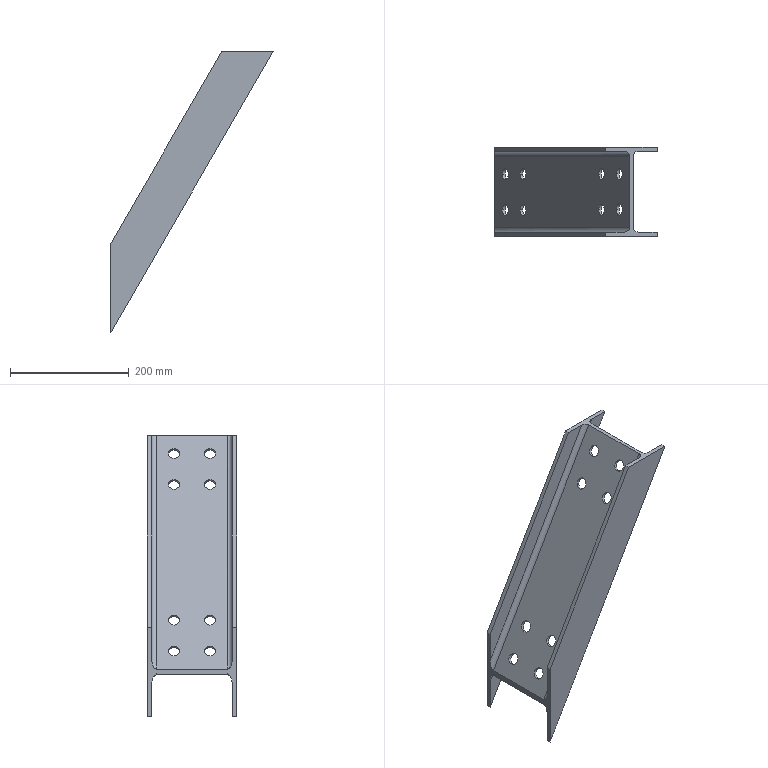Part | STEP file | 粉仓Diagonal Brace梁3-1_Default<As Machined> | 1 solid | 34 faces | box 273.301 x 150 x 473.372 mm | volume 809730 mm3 | cylinder 20 | plane 14 | commonest cylinder face diameters 19 x16 16 x4